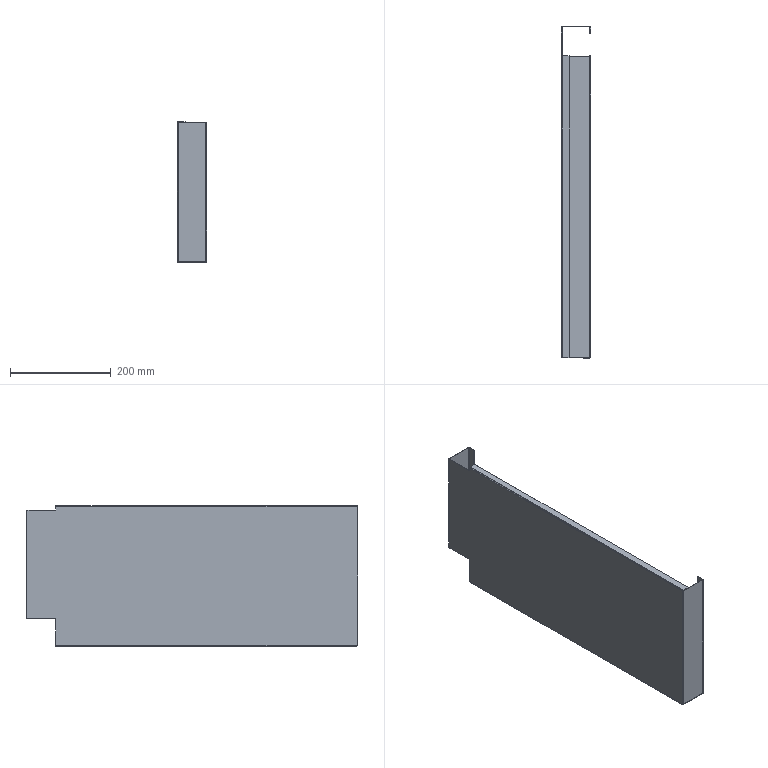Part | SolidWorks | features EdgeFlange 3, FlatPattern 1, ICE 1, SMBaseFlange 1, SheetMetal 1 | 1 solid | 69 faces | box 57.6 x 657.6 x 278.8 mm | volume 314044 mm3 | plane 51 | cylinder 14 | spline 4 | commonest cylinder face diameters 0.9 x7 3.3 x7